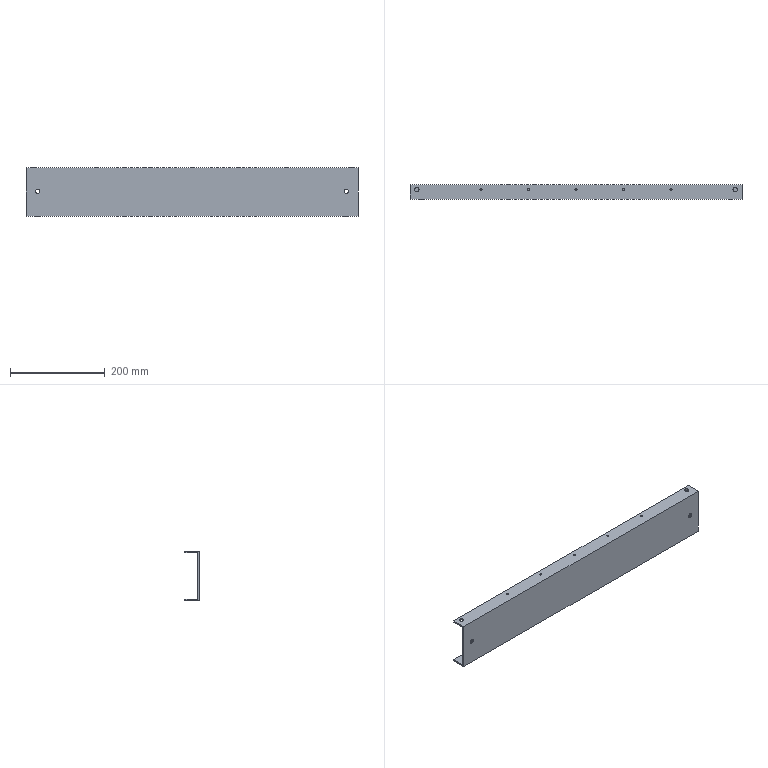Part | SolidWorks | features BaseBody 1 | 1 solid | 32 faces | box 699 x 30 x 103 mm | volume 327650 mm3 | cylinder 22 | plane 10 | commonest cylinder face diameters 4.4 x10 9.1 x8 11 x4
STEP:
#1=CARTESIAN_POINT('',(871.946,-4400.973,890.421));
#2=VERTEX_POINT('',#1);
#3=CARTESIAN_POINT('',(871.946,-4400.973,899.521));
#4=VERTEX_POINT('',#3);
#5=CARTESIAN_POINT('',(871.946,-4400.973,894.971));
#6=DIRECTION('',(0.,1.,0.));
#7=DIRECTION('',(0.,0.,1.));
#8=AXIS2_PLACEMENT_3D('',#5,#6,#7);
#9=CIRCLE('',#8,4.55);
#10=EDGE_CURVE('',#2,#4,#9,.T.);
#11=ORIENTED_EDGE('',*,*,#10,.F.);
#12=CARTESIAN_POINT('',(871.946,-4397.973,890.421));
#13=VERTEX_POINT('',#12);
#14=CARTESIAN_POINT('',(871.946,-4381.737,890.421));
#15=DIRECTION('',(0.,1.,0.));
#16=VECTOR('',#15,1000.);
#17=LINE('',#14,#16);
#18=EDGE_CURVE('',#2,#13,#17,.T.);
#19=ORIENTED_EDGE('',*,*,#18,.T.);
#20=CARTESIAN_POINT('',(871.946,-4397.973,899.521));
#21=VERTEX_POINT('',#20);
#22=CARTESIAN_POINT('',(871.946,-4397.973,894.971));
#23=DIRECTION('',(0.,-1.,0.));
#24=DIRECTION('',(0.,0.,1.));
#25=AXIS2_PLACEMENT_3D('',#22,#23,#24);
#26=CIRCLE('',#25,4.55);
#27=EDGE_CURVE('',#21,#13,#26,.T.);
#28=ORIENTED_EDGE('',*,*,#27,.F.);
#29=CARTESIAN_POINT('',(871.946,-4381.737,899.521));
#30=DIRECTION('',(0.,1.,0.));
#31=VECTOR('',#30,1000.);
#32=LINE('',#29,#31);
#33=EDGE_CURVE('',#4,#21,#32,.T.);
#34=ORIENTED_EDGE('',*,*,#33,.F.);
#35=EDGE_LOOP('',(#11,#19,#28,#34));
#36=FACE_OUTER_BOUND('',#35,.T.);
#37=CARTESIAN_POINT('',(871.946,-4381.737,894.971));
#38=DIRECTION('',(0.,1.,0.));
#39=DIRECTION('',(0.,0.,1.));
#40=AXIS2_PLACEMENT_3D('',#37,#38,#39);
#41=CYLINDRICAL_SURFACE('',#40,4.55);
#42=ADVANCED_FACE('',(#36),#41,.F.);
#43=CARTESIAN_POINT('',(221.946,-4397.973,899.521));
#44=VERTEX_POINT('',#43);
#45=CARTESIAN_POINT('',(221.946,-4397.973,890.421));
#46=VERTEX_POINT('',#45);
#47=CARTESIAN_POINT('',(221.946,-4397.973,894.971));
#48=DIRECTION('',(0.,-1.,0.));
#49=DIRECTION('',(0.,0.,-1.));
#50=AXIS2_PLACEMENT_3D('',#47,#48,#49);
#51=CIRCLE('',#50,4.55);
#52=EDGE_CURVE('',#44,#46,#51,.T.);
#53=ORIENTED_EDGE('',*,*,#52,.F.);
#54=CARTESIAN_POINT('',(221.946,-4400.973,899.521));
#55=VERTEX_POINT('',#54);
#56=CARTESIAN_POINT('',(221.946,-4381.737,899.521));
#57=DIRECTION('',(0.,-1.,0.));
#58=VECTOR('',#57,1000.);
#59=LINE('',#56,#58);
#60=EDGE_CURVE('',#44,#55,#59,.T.);
#61=ORIENTED_EDGE('',*,*,#60,.T.);
#62=CARTESIAN_POINT('',(221.946,-4400.973,890.421));
#63=VERTEX_POINT('',#62);
#64=CARTESIAN_POINT('',(221.946,-4400.973,894.971));
#65=DIRECTION('',(0.,1.,0.));
#66=DIRECTION('',(0.,0.,-1.));
#67=AXIS2_PLACEMENT_3D('',#64,#65,#66);
#68=CIRCLE('',#67,4.55);
#69=EDGE_CURVE('',#63,#55,#68,.T.);
#70=ORIENTED_EDGE('',*,*,#69,.F.);
#71=CARTESIAN_POINT('',(221.946,-4381.737,890.421));
#72=DIRECTION('',(0.,-1.,0.));
#73=VECTOR('',#72,1000.);
#74=LINE('',#71,#73);
#75=EDGE_CURVE('',#46,#63,#74,.T.);
#76=ORIENTED_EDGE('',*,*,#75,.F.);
#77=EDGE_LOOP('',(#53,#61,#70,#76));
#78=FACE_OUTER_BOUND('',#77,.T.);
#79=CARTESIAN_POINT('',(221.946,-4381.737,894.971));
#80=DIRECTION('',(0.,-1.,0.));
#81=DIRECTION('',(0.,0.,-1.));
#82=AXIS2_PLACEMENT_3D('',#79,#80,#81);
#83=CYLINDRICAL_SURFACE('',#82,4.55);
#84=ADVANCED_FACE('',(#78),#83,.F.);
#85=CARTESIAN_POINT('',(886.496,-4380.973,944.971));
#86=VERTEX_POINT('',#85);
#87=CARTESIAN_POINT('',(877.396,-4380.973,944.971));
#88=VERTEX_POINT('',#87);
#89=CARTESIAN_POINT('',(881.946,-4380.973,944.971));
#90=DIRECTION('',(0.,0.,-1.));
#91=DIRECTION('',(-1.,0.,0.));
#92=AXIS2_PLACEMENT_3D('',#89,#90,#91);
#93=CIRCLE('',#92,4.55);
#94=EDGE_CURVE('',#86,#88,#93,.T.);
#95=ORIENTED_EDGE('',*,*,#94,.F.);
#96=CARTESIAN_POINT('',(886.496,-4380.973,941.971));
#97=VERTEX_POINT('',#96);
#98=CARTESIAN_POINT('',(886.496,-4380.973,946.133));
#99=DIRECTION('',(0.,0.,-1.));
#100=VECTOR('',#99,1000.);
#101=LINE('',#98,#100);
#102=EDGE_CURVE('',#86,#97,#101,.T.);
#103=ORIENTED_EDGE('',*,*,#102,.T.);
#104=CARTESIAN_POINT('',(877.396,-4380.973,941.971));
#105=VERTEX_POINT('',#104);
#106=CARTESIAN_POINT('',(881.946,-4380.973,941.971));
#107=DIRECTION('',(0.,0.,1.));
#108=DIRECTION('',(-1.,0.,0.));
#109=AXIS2_PLACEMENT_3D('',#106,#107,#108);
#110=CIRCLE('',#109,4.55);
#111=EDGE_CURVE('',#105,#97,#110,.T.);
#112=ORIENTED_EDGE('',*,*,#111,.F.);
#113=CARTESIAN_POINT('',(877.396,-4380.973,946.133));
#114=DIRECTION('',(0.,0.,-1.));
#115=VECTOR('',#114,1000.);
#116=LINE('',#113,#115);
#117=EDGE_CURVE('',#88,#105,#116,.T.);
#118=ORIENTED_EDGE('',*,*,#117,.F.);
#119=EDGE_LOOP('',(#95,#103,#112,#118));
#120=FACE_OUTER_BOUND('',#119,.T.);
#121=CARTESIAN_POINT('',(881.946,-4380.973,946.133));
#122=DIRECTION('',(0.,0.,-1.));
#123=DIRECTION('',(-1.,0.,0.));
#124=AXIS2_PLACEMENT_3D('',#121,#122,#123);
#125=CYLINDRICAL_SURFACE('',#124,4.55);
#126=ADVANCED_FACE('',(#120),#125,.F.);
#127=CARTESIAN_POINT('',(207.396,-4380.973,941.971));
#128=VERTEX_POINT('',#127);
#129=CARTESIAN_POINT('',(216.496,-4380.973,941.971));
#130=VERTEX_POINT('',#129);
#131=CARTESIAN_POINT('',(211.946,-4380.973,941.971));
#132=DIRECTION('',(0.,0.,1.));
#133=DIRECTION('',(1.,0.,0.));
#134=AXIS2_PLACEMENT_3D('',#131,#132,#133);
#135=CIRCLE('',#134,4.55);
#136=EDGE_CURVE('',#128,#130,#135,.T.);
#137=ORIENTED_EDGE('',*,*,#136,.F.);
#138=CARTESIAN_POINT('',(207.396,-4380.973,944.971));
#139=VERTEX_POINT('',#138);
#140=CARTESIAN_POINT('',(207.396,-4380.973,946.133));
#141=DIRECTION('',(0.,0.,1.));
#142=VECTOR('',#141,1000.);
#143=LINE('',#140,#142);
#144=EDGE_CURVE('',#128,#139,#143,.T.);
#145=ORIENTED_EDGE('',*,*,#144,.T.);
#146=CARTESIAN_POINT('',(216.496,-4380.973,944.971));
#147=VERTEX_POINT('',#146);
#148=CARTESIAN_POINT('',(211.946,-4380.973,944.971));
#149=DIRECTION('',(0.,0.,-1.));
#150=DIRECTION('',(1.,0.,0.));
#151=AXIS2_PLACEMENT_3D('',#148,#149,#150);
#152=CIRCLE('',#151,4.55);
#153=EDGE_CURVE('',#147,#139,#152,.T.);
#154=ORIENTED_EDGE('',*,*,#153,.F.);
#155=CARTESIAN_POINT('',(216.496,-4380.973,946.133));
#156=DIRECTION('',(0.,0.,1.));
#157=VECTOR('',#156,1000.);
#158=LINE('',#155,#157);
#159=EDGE_CURVE('',#130,#147,#158,.T.);
#160=ORIENTED_EDGE('',*,*,#159,.F.);
#161=EDGE_LOOP('',(#137,#145,#154,#160));
#162=FACE_OUTER_BOUND('',#161,.T.);
#163=CARTESIAN_POINT('',(211.946,-4380.973,946.133));
#164=DIRECTION('',(0.,0.,1.));
#165=DIRECTION('',(1.,0.,0.));
#166=AXIS2_PLACEMENT_3D('',#163,#164,#165);
#167=CYLINDRICAL_SURFACE('',#166,4.55);
#168=ADVANCED_FACE('',(#162),#167,.F.);
#169=CARTESIAN_POINT('',(544.746,-4380.973,941.971));
#170=VERTEX_POINT('',#169);
#171=CARTESIAN_POINT('',(549.146,-4380.973,941.971));
#172=VERTEX_POINT('',#171);
#173=CARTESIAN_POINT('',(546.946,-4380.973,941.971));
#174=DIRECTION('',(0.,0.,1.));
#175=DIRECTION('',(1.,0.,0.));
#176=AXIS2_PLACEMENT_3D('',#173,#174,#175);
#177=CIRCLE('',#176,2.2);
#178=EDGE_CURVE('',#170,#172,#177,.T.);
#179=ORIENTED_EDGE('',*,*,#178,.F.);
#180=CARTESIAN_POINT('',(544.746,-4380.973,944.971));
#181=VERTEX_POINT('',#180);
#182=CARTESIAN_POINT('',(544.746,-4380.973,945.024));
#183=DIRECTION('',(0.,0.,1.));
#184=VECTOR('',#183,1000.);
#185=LINE('',#182,#184);
#186=EDGE_CURVE('',#170,#181,#185,.T.);
#187=ORIENTED_EDGE('',*,*,#186,.T.);
#188=CARTESIAN_POINT('',(549.146,-4380.973,944.971));
#189=VERTEX_POINT('',#188);
#190=CARTESIAN_POINT('',(546.946,-4380.973,944.971));
#191=DIRECTION('',(0.,0.,-1.));
#192=DIRECTION('',(1.,0.,0.));
#193=AXIS2_PLACEMENT_3D('',#190,#191,#192);
#194=CIRCLE('',#193,2.2);
#195=EDGE_CURVE('',#189,#181,#194,.T.);
#196=ORIENTED_EDGE('',*,*,#195,.F.);
#197=CARTESIAN_POINT('',(549.146,-4380.973,945.024));
#198=DIRECTION('',(0.,0.,1.));
#199=VECTOR('',#198,1000.);
#200=LINE('',#197,#199);
#201=EDGE_CURVE('',#172,#189,#200,.T.);
#202=ORIENTED_EDGE('',*,*,#201,.F.);
#203=EDGE_LOOP('',(#179,#187,#196,#202));
#204=FACE_OUTER_BOUND('',#203,.T.);
#205=CARTESIAN_POINT('',(546.946,-4380.973,945.024));
#206=DIRECTION('',(0.,0.,1.));
#207=DIRECTION('',(1.,0.,0.));
#208=AXIS2_PLACEMENT_3D('',#205,#206,#207);
#209=CYLINDRICAL_SURFACE('',#208,2.2);
#210=ADVANCED_FACE('',(#204),#209,.F.);
#211=CARTESIAN_POINT('',(344.746,-4380.973,941.971));
#212=VERTEX_POINT('',#211);
#213=CARTESIAN_POINT('',(349.146,-4380.973,941.971));
#214=VERTEX_POINT('',#213);
#215=CARTESIAN_POINT('',(346.946,-4380.973,941.971));
#216=DIRECTION('',(0.,0.,1.));
#217=DIRECTION('',(1.,0.,0.));
#218=AXIS2_PLACEMENT_3D('',#215,#216,#217);
#219=CIRCLE('',#218,2.2);
#220=EDGE_CURVE('',#212,#214,#219,.T.);
#221=ORIENTED_EDGE('',*,*,#220,.F.);
#222=CARTESIAN_POINT('',(344.746,-4380.973,944.971));
#223=VERTEX_POINT('',#222);
#224=CARTESIAN_POINT('',(344.746,-4380.973,945.024));
#225=DIRECTION('',(0.,0.,1.));
#226=VECTOR('',#225,1000.);
#227=LINE('',#224,#226);
#228=EDGE_CURVE('',#212,#223,#227,.T.);
#229=ORIENTED_EDGE('',*,*,#228,.T.);
#230=CARTESIAN_POINT('',(349.146,-4380.973,944.971));
#231=VERTEX_POINT('',#230);
#232=CARTESIAN_POINT('',(346.946,-4380.973,944.971));
#233=DIRECTION('',(0.,0.,-1.));
#234=DIRECTION('',(1.,0.,0.));
#235=AXIS2_PLACEMENT_3D('',#232,#233,#234);
#236=CIRCLE('',#235,2.2);
#237=EDGE_CURVE('',#231,#223,#236,.T.);
#238=ORIENTED_EDGE('',*,*,#237,.F.);
#239=CARTESIAN_POINT('',(349.146,-4380.973,945.024));
#240=DIRECTION('',(0.,0.,1.));
#241=VECTOR('',#240,1000.);
#242=LINE('',#239,#241);
#243=EDGE_CURVE('',#214,#231,#242,.T.);
#244=ORIENTED_EDGE('',*,*,#243,.F.);
#245=EDGE_LOOP('',(#221,#229,#238,#244));
#246=FACE_OUTER_BOUND('',#245,.T.);
#247=CARTESIAN_POINT('',(346.946,-4380.973,945.024));
#248=DIRECTION('',(0.,0.,1.));
#249=DIRECTION('',(1.,0.,0.));
#250=AXIS2_PLACEMENT_3D('',#247,#248,#249);
#251=CYLINDRICAL_SURFACE('',#250,2.2);
#252=ADVANCED_FACE('',(#246),#251,.F.);
#253=CARTESIAN_POINT('',(649.146,-4380.973,944.971));
#254=VERTEX_POINT('',#253);
#255=CARTESIAN_POINT('',(644.746,-4380.973,944.971));
#256=VERTEX_POINT('',#255);
#257=CARTESIAN_POINT('',(646.946,-4380.973,944.971));
#258=DIRECTION('',(0.,0.,-1.));
#259=DIRECTION('',(-1.,0.,0.));
#260=AXIS2_PLACEMENT_3D('',#257,#258,#259);
#261=CIRCLE('',#260,2.2);
#262=EDGE_CURVE('',#254,#256,#261,.T.);
#263=ORIENTED_EDGE('',*,*,#262,.F.);
#264=CARTESIAN_POINT('',(649.146,-4380.973,941.971));
#265=VERTEX_POINT('',#264);
#266=CARTESIAN_POINT('',(649.146,-4380.973,945.024));
#267=DIRECTION('',(0.,0.,-1.));
#268=VECTOR('',#267,1000.);
#269=LINE('',#266,#268);
#270=EDGE_CURVE('',#254,#265,#269,.T.);
#271=ORIENTED_EDGE('',*,*,#270,.T.);
#272=CARTESIAN_POINT('',(644.746,-4380.973,941.971));
#273=VERTEX_POINT('',#272);
#274=CARTESIAN_POINT('',(646.946,-4380.973,941.971));
#275=DIRECTION('',(0.,0.,1.));
#276=DIRECTION('',(-1.,0.,0.));
#277=AXIS2_PLACEMENT_3D('',#274,#275,#276);
#278=CIRCLE('',#277,2.2);
#279=EDGE_CURVE('',#273,#265,#278,.T.);
#280=ORIENTED_EDGE('',*,*,#279,.F.);
#281=CARTESIAN_POINT('',(644.746,-4380.973,945.024));
#282=DIRECTION('',(0.,0.,-1.));
#283=VECTOR('',#282,1000.);
#284=LINE('',#281,#283);
#285=EDGE_CURVE('',#256,#273,#284,.T.);
#286=ORIENTED_EDGE('',*,*,#285,.F.);
#287=EDGE_LOOP('',(#263,#271,#280,#286));
#288=FACE_OUTER_BOUND('',#287,.T.);
#289=CARTESIAN_POINT('',(646.946,-4380.973,945.024));
#290=DIRECTION('',(0.,0.,-1.));
#291=DIRECTION('',(-1.,0.,0.));
#292=AXIS2_PLACEMENT_3D('',#289,#290,#291);
#293=CYLINDRICAL_SURFACE('',#292,2.2);
#294=ADVANCED_FACE('',(#288),#293,.F.);
#295=CARTESIAN_POINT('',(749.146,-4380.973,944.971));
#296=VERTEX_POINT('',#295);
#297=CARTESIAN_POINT('',(744.746,-4380.973,944.971));
#298=VERTEX_POINT('',#297);
#299=CARTESIAN_POINT('',(746.946,-4380.973,944.971));
#300=DIRECTION('',(0.,0.,-1.));
#301=DIRECTION('',(-1.,0.,0.));
#302=AXIS2_PLACEMENT_3D('',#299,#300,#301);
#303=CIRCLE('',#302,2.2);
#304=EDGE_CURVE('',#296,#298,#303,.T.);
#305=ORIENTED_EDGE('',*,*,#304,.F.);
#306=CARTESIAN_POINT('',(749.146,-4380.973,941.971));
#307=VERTEX_POINT('',#306);
#308=CARTESIAN_POINT('',(749.146,-4380.973,945.024));
#309=DIRECTION('',(0.,0.,-1.));
#310=VECTOR('',#309,1000.);
#311=LINE('',#308,#310);
#312=EDGE_CURVE('',#296,#307,#311,.T.);
#313=ORIENTED_EDGE('',*,*,#312,.T.);
#314=CARTESIAN_POINT('',(744.746,-4380.973,941.971));
#315=VERTEX_POINT('',#314);
#316=CARTESIAN_POINT('',(746.946,-4380.973,941.971));
#317=DIRECTION('',(0.,0.,1.));
#318=DIRECTION('',(-1.,0.,0.));
#319=AXIS2_PLACEMENT_3D('',#316,#317,#318);
#320=CIRCLE('',#319,2.2);
#321=EDGE_CURVE('',#315,#307,#320,.T.);
#322=ORIENTED_EDGE('',*,*,#321,.F.);
#323=CARTESIAN_POINT('',(744.746,-4380.973,945.024));
#324=DIRECTION('',(0.,0.,-1.));
#325=VECTOR('',#324,1000.);
#326=LINE('',#323,#325);
#327=EDGE_CURVE('',#298,#315,#326,.T.);
#328=ORIENTED_EDGE('',*,*,#327,.F.);
#329=EDGE_LOOP('',(#305,#313,#322,#328));
#330=FACE_OUTER_BOUND('',#329,.T.);
#331=CARTESIAN_POINT('',(746.946,-4380.973,945.024));
#332=DIRECTION('',(0.,0.,-1.));
#333=DIRECTION('',(-1.,0.,0.));
#334=AXIS2_PLACEMENT_3D('',#331,#332,#333);
#335=CYLINDRICAL_SURFACE('',#334,2.2);
#336=ADVANCED_FACE('',(#330),#335,.F.);
#337=CARTESIAN_POINT('',(444.746,-4380.973,941.971));
#338=VERTEX_POINT('',#337);
#339=CARTESIAN_POINT('',(449.146,-4380.973,941.971));
#340=VERTEX_POINT('',#339);
#341=CARTESIAN_POINT('',(446.946,-4380.973,941.971));
#342=DIRECTION('',(0.,0.,1.));
#343=DIRECTION('',(1.,0.,0.));
#344=AXIS2_PLACEMENT_3D('',#341,#342,#343);
#345=CIRCLE('',#344,2.2);
#346=EDGE_CURVE('',#338,#340,#345,.T.);
#347=ORIENTED_EDGE('',*,*,#346,.F.);
#348=CARTESIAN_POINT('',(444.746,-4380.973,944.971));
#349=VERTEX_POINT('',#348);
#350=CARTESIAN_POINT('',(444.746,-4380.973,945.024));
#351=DIRECTION('',(0.,0.,1.));
#352=VECTOR('',#351,1000.);
#353=LINE('',#350,#352);
#354=EDGE_CURVE('',#338,#349,#353,.T.);
#355=ORIENTED_EDGE('',*,*,#354,.T.);
#356=CARTESIAN_POINT('',(449.146,-4380.973,944.971));
#357=VERTEX_POINT('',#356);
#358=CARTESIAN_POINT('',(446.946,-4380.973,944.971));
#359=DIRECTION('',(0.,0.,-1.));
#360=DIRECTION('',(1.,0.,0.));
#361=AXIS2_PLACEMENT_3D('',#358,#359,#360);
#362=CIRCLE('',#361,2.2);
#363=EDGE_CURVE('',#357,#349,#362,.T.);
#364=ORIENTED_EDGE('',*,*,#363,.F.);
#365=CARTESIAN_POINT('',(449.146,-4380.973,945.024));
#366=DIRECTION('',(0.,0.,1.));
#367=VECTOR('',#366,1000.);
#368=LINE('',#365,#367);
#369=EDGE_CURVE('',#340,#357,#368,.T.);
#370=ORIENTED_EDGE('',*,*,#369,.F.);
#371=EDGE_LOOP('',(#347,#355,#364,#370));
#372=FACE_OUTER_BOUND('',#371,.T.);
#373=CARTESIAN_POINT('',(446.946,-4380.973,945.024));
#374=DIRECTION('',(0.,0.,1.));
#375=DIRECTION('',(1.,0.,0.));
#376=AXIS2_PLACEMENT_3D('',#373,#374,#375);
#377=CYLINDRICAL_SURFACE('',#376,2.2);
#378=ADVANCED_FACE('',(#372),#377,.F.);
#379=CARTESIAN_POINT('',(216.446,-4380.973,841.971));
#380=VERTEX_POINT('',#379);
#381=CARTESIAN_POINT('',(227.446,-4380.973,841.971));
#382=VERTEX_POINT('',#381);
#383=CARTESIAN_POINT('',(221.946,-4380.973,841.971));
#384=DIRECTION('',(0.,0.,1.));
#385=DIRECTION('',(1.,0.,0.));
#386=AXIS2_PLACEMENT_3D('',#383,#384,#385);
#387=CIRCLE('',#386,5.5);
#388=EDGE_CURVE('',#380,#382,#387,.T.);
#389=ORIENTED_EDGE('',*,*,#388,.F.);
#390=CARTESIAN_POINT('',(216.446,-4380.973,844.971));
#391=VERTEX_POINT('',#390);
#392=CARTESIAN_POINT('',(216.446,-4380.973,832.653));
#393=DIRECTION('',(0.,0.,1.));
#394=VECTOR('',#393,1000.);
#395=LINE('',#392,#394);
#396=EDGE_CURVE('',#380,#391,#395,.T.);
#397=ORIENTED_EDGE('',*,*,#396,.T.);
#398=CARTESIAN_POINT('',(227.446,-4380.973,844.971));
#399=VERTEX_POINT('',#398);
#400=CARTESIAN_POINT('',(221.946,-4380.973,844.971));
#401=DIRECTION('',(0.,0.,-1.));
#402=DIRECTION('',(1.,0.,0.));
#403=AXIS2_PLACEMENT_3D('',#400,#401,#402);
#404=CIRCLE('',#403,5.5);
#405=EDGE_CURVE('',#399,#391,#404,.T.);
#406=ORIENTED_EDGE('',*,*,#405,.F.);
#407=CARTESIAN_POINT('',(227.446,-4380.973,832.653));
#408=DIRECTION('',(0.,0.,1.));
#409=VECTOR('',#408,1000.);
#410=LINE('',#407,#409);
#411=EDGE_CURVE('',#382,#399,#410,.T.);
#412=ORIENTED_EDGE('',*,*,#411,.F.);
#413=EDGE_LOOP('',(#389,#397,#406,#412));
#414=FACE_OUTER_BOUND('',#413,.T.);
#415=CARTESIAN_POINT('',(221.946,-4380.973,832.653));
#416=DIRECTION('',(0.,0.,1.));
#417=DIRECTION('',(1.,0.,0.));
#418=AXIS2_PLACEMENT_3D('',#415,#416,#417);
#419=CYLINDRICAL_SURFACE('',#418,5.5);
#420=ADVANCED_FACE('',(#414),#419,.F.);
#421=CARTESIAN_POINT('',(877.446,-4380.973,844.971));
#422=VERTEX_POINT('',#421);
#423=CARTESIAN_POINT('',(866.446,-4380.973,844.971));
#424=VERTEX_POINT('',#423);
#425=CARTESIAN_POINT('',(871.946,-4380.973,844.971));
#426=DIRECTION('',(0.,0.,-1.));
#427=DIRECTION('',(-1.,0.,0.));
#428=AXIS2_PLACEMENT_3D('',#425,#426,#427);
#429=CIRCLE('',#428,5.5);
#430=EDGE_CURVE('',#422,#424,#429,.T.);
#431=ORIENTED_EDGE('',*,*,#430,.F.);
#432=CARTESIAN_POINT('',(877.446,-4380.973,841.971));
#433=VERTEX_POINT('',#432);
#434=CARTESIAN_POINT('',(877.446,-4380.973,832.653));
#435=DIRECTION('',(0.,0.,-1.));
#436=VECTOR('',#435,1000.);
#437=LINE('',#434,#436);
#438=EDGE_CURVE('',#422,#433,#437,.T.);
#439=ORIENTED_EDGE('',*,*,#438,.T.);
#440=CARTESIAN_POINT('',(866.446,-4380.973,841.971));
#441=VERTEX_POINT('',#440);
#442=CARTESIAN_POINT('',(871.946,-4380.973,841.971));
#443=DIRECTION('',(0.,0.,1.));
#444=DIRECTION('',(-1.,0.,0.));
#445=AXIS2_PLACEMENT_3D('',#442,#443,#444);
#446=CIRCLE('',#445,5.5);
#447=EDGE_CURVE('',#441,#433,#446,.T.);
#448=ORIENTED_EDGE('',*,*,#447,.F.);
#449=CARTESIAN_POINT('',(866.446,-4380.973,832.653));
#450=DIRECTION('',(0.,0.,-1.));
#451=VECTOR('',#450,1000.);
#452=LINE('',#449,#451);
#453=EDGE_CURVE('',#424,#441,#452,.T.);
#454=ORIENTED_EDGE('',*,*,#453,.F.);
#455=EDGE_LOOP('',(#431,#439,#448,#454));
#456=FACE_OUTER_BOUND('',#455,.T.);
#457=CARTESIAN_POINT('',(871.946,-4380.973,832.653));
#458=DIRECTION('',(0.,0.,-1.));
#459=DIRECTION('',(-1.,0.,0.));
#460=AXIS2_PLACEMENT_3D('',#457,#458,#459);
#461=CYLINDRICAL_SURFACE('',#460,5.5);
#462=ADVANCED_FACE('',(#456),#461,.F.);
#463=CARTESIAN_POINT('',(896.446,-4400.973,841.971));
#464=VERTEX_POINT('',#463);
#465=CARTESIAN_POINT('',(896.446,-4400.973,944.971));
#466=VERTEX_POINT('',#465);
#467=CARTESIAN_POINT('',(896.446,-4400.973,944.971));
#468=DIRECTION('',(0.,0.,1.));
#469=VECTOR('',#468,1000.);
#470=LINE('',#467,#469);
#471=EDGE_CURVE('',#464,#466,#470,.T.);
#472=ORIENTED_EDGE('',*,*,#471,.T.);
#473=CARTESIAN_POINT('',(197.446,-4400.973,944.971));
#474=VERTEX_POINT('',#473);
#475=CARTESIAN_POINT('',(896.446,-4400.973,944.971));
#476=DIRECTION('',(-1.,0.,0.));
#477=VECTOR('',#476,1000.);
#478=LINE('',#475,#477);
#479=EDGE_CURVE('',#466,#474,#478,.T.);
#480=ORIENTED_EDGE('',*,*,#479,.T.);
#481=CARTESIAN_POINT('',(197.446,-4400.973,841.971));
#482=VERTEX_POINT('',#481);
#483=CARTESIAN_POINT('',(197.446,-4400.973,944.971));
#484=DIRECTION('',(0.,0.,-1.));
#485=VECTOR('',#484,1000.);
#486=LINE('',#483,#485);
#487=EDGE_CURVE('',#474,#482,#486,.T.);
#488=ORIENTED_EDGE('',*,*,#487,.T.);
#489=CARTESIAN_POINT('',(896.446,-4400.973,841.971));
#490=DIRECTION('',(1.,0.,0.));
#491=VECTOR('',#490,1000.);
#492=LINE('',#489,#491);
#493=EDGE_CURVE('',#482,#464,#492,.T.);
#494=ORIENTED_EDGE('',*,*,#493,.T.);
#495=EDGE_LOOP('',(#472,#480,#488,#494));
#496=FACE_OUTER_BOUND('',#495,.T.);
#497=CARTESIAN_POINT('',(871.946,-4400.973,894.971));
#498=DIRECTION('',(0.,1.,0.));
#499=DIRECTION('',(0.,0.,1.));
#500=AXIS2_PLACEMENT_3D('',#497,#498,#499);
#501=CIRCLE('',#500,4.55);
#502=EDGE_CURVE('',#4,#2,#501,.T.);
#503=ORIENTED_EDGE('',*,*,#502,.T.);
#504=ORIENTED_EDGE('',*,*,#10,.T.);
#505=EDGE_LOOP('',(#503,#504));
#506=FACE_BOUND('',#505,.T.);
#507=ORIENTED_EDGE('',*,*,#69,.T.);
#508=CARTESIAN_POINT('',(221.946,-4400.973,894.971));
#509=DIRECTION('',(0.,1.,0.));
#510=DIRECTION('',(0.,0.,-1.));
#511=AXIS2_PLACEMENT_3D('',#508,#509,#510);
#512=CIRCLE('',#511,4.55);
#513=EDGE_CURVE('',#55,#63,#512,.T.);
#514=ORIENTED_EDGE('',*,*,#513,.T.);
#515=EDGE_LOOP('',(#507,#514));
#516=FACE_BOUND('',#515,.T.);
#517=CARTESIAN_POINT('',(896.446,-4400.973,944.971));
#518=DIRECTION('',(0.,-1.,0.));
#519=DIRECTION('',(0.,0.,-1.));
#520=AXIS2_PLACEMENT_3D('',#517,#518,#519);
#521=PLANE('',#520);
#522=ADVANCED_FACE('',(#496,#506,#516),#521,.T.);
#523=CARTESIAN_POINT('',(896.446,-4370.973,944.971));
#524=VERTEX_POINT('',#523);
#525=CARTESIAN_POINT('',(896.446,-4375.973,944.971));
#526=DIRECTION('',(0.,1.,0.));
#527=VECTOR('',#526,1000.);
#528=LINE('',#525,#527);
#529=EDGE_CURVE('',#466,#524,#528,.T.);
#530=ORIENTED_EDGE('',*,*,#529,.T.);
#531=CARTESIAN_POINT('',(197.446,-4370.973,944.971));
#532=VERTEX_POINT('',#531);
#533=CARTESIAN_POINT('',(896.446,-4370.973,944.971));
#534=DIRECTION('',(-1.,0.,0.));
#535=VECTOR('',#534,1000.);
#536=LINE('',#533,#535);
#537=EDGE_CURVE('',#524,#532,#536,.T.);
#538=ORIENTED_EDGE('',*,*,#537,.T.);
#539=CARTESIAN_POINT('',(197.446,-4375.973,944.971));
#540=DIRECTION('',(0.,-1.,0.));
#541=VECTOR('',#540,1000.);
#542=LINE('',#539,#541);
#543=EDGE_CURVE('',#532,#474,#542,.T.);
#544=ORIENTED_EDGE('',*,*,#543,.T.);
#545=ORIENTED_EDGE('',*,*,#479,.F.);
#546=EDGE_LOOP('',(#530,#538,#544,#545));
#547=FACE_OUTER_BOUND('',#546,.T.);
#548=CARTESIAN_POINT('',(881.946,-4380.973,944.971));
#549=DIRECTION('',(0.,0.,-1.));
#550=DIRECTION('',(-1.,0.,0.));
#551=AXIS2_PLACEMENT_3D('',#548,#549,#550);
#552=CIRCLE('',#551,4.55);
#553=EDGE_CURVE('',#88,#86,#552,.T.);
#554=ORIENTED_EDGE('',*,*,#553,.T.);
#555=ORIENTED_EDGE('',*,*,#94,.T.);
#556=EDGE_LOOP('',(#554,#555));
#557=FACE_BOUND('',#556,.T.);
#558=ORIENTED_EDGE('',*,*,#153,.T.);
#559=CARTESIAN_POINT('',(211.946,-4380.973,944.971));
#560=DIRECTION('',(0.,0.,-1.));
#561=DIRECTION('',(1.,0.,0.));
#562=AXIS2_PLACEMENT_3D('',#559,#560,#561);
#563=CIRCLE('',#562,4.55);
#564=EDGE_CURVE('',#139,#147,#563,.T.);
#565=ORIENTED_EDGE('',*,*,#564,.T.);
#566=EDGE_LOOP('',(#558,#565));
#567=FACE_BOUND('',#566,.T.);
#568=ORIENTED_EDGE('',*,*,#195,.T.);
#569=CARTESIAN_POINT('',(546.946,-4380.973,944.971));
#570=DIRECTION('',(0.,0.,-1.));
#571=DIRECTION('',(1.,0.,0.));
#572=AXIS2_PLACEMENT_3D('',#569,#570,#571);
#573=CIRCLE('',#572,2.2);
#574=EDGE_CURVE('',#181,#189,#573,.T.);
#575=ORIENTED_EDGE('',*,*,#574,.T.);
#576=EDGE_LOOP('',(#568,#575));
#577=FACE_BOUND('',#576,.T.);
#578=ORIENTED_EDGE('',*,*,#237,.T.);
#579=CARTESIAN_POINT('',(346.946,-4380.973,944.971));
#580=DIRECTION('',(0.,0.,-1.));
#581=DIRECTION('',(1.,0.,0.));
#582=AXIS2_PLACEMENT_3D('',#579,#580,#581);
#583=CIRCLE('',#582,2.2);
#584=EDGE_CURVE('',#223,#231,#583,.T.);
#585=ORIENTED_EDGE('',*,*,#584,.T.);
#586=EDGE_LOOP('',(#578,#585));
#587=FACE_BOUND('',#586,.T.);
#588=CARTESIAN_POINT('',(646.946,-4380.973,944.971));
#589=DIRECTION('',(0.,0.,-1.));
#590=DIRECTION('',(-1.,0.,0.));
#591=AXIS2_PLACEMENT_3D('',#588,#589,#590);
#592=CIRCLE('',#591,2.2);
#593=EDGE_CURVE('',#256,#254,#592,.T.);
#594=ORIENTED_EDGE('',*,*,#593,.T.);
#595=ORIENTED_EDGE('',*,*,#262,.T.);
#596=EDGE_LOOP('',(#594,#595));
#597=FACE_BOUND('',#596,.T.);
#598=CARTESIAN_POINT('',(746.946,-4380.973,944.971));
#599=DIRECTION('',(0.,0.,-1.));
#600=DIRECTION('',(-1.,0.,0.));
#601=AXIS2_PLACEMENT_3D('',#598,#599,#600);
#602=CIRCLE('',#601,2.2);
#603=EDGE_CURVE('',#298,#296,#602,.T.);
#604=ORIENTED_EDGE('',*,*,#603,.T.);
#605=ORIENTED_EDGE('',*,*,#304,.T.);
#606=EDGE_LOOP('',(#604,#605));
#607=FACE_BOUND('',#606,.T.);
#608=ORIENTED_EDGE('',*,*,#363,.T.);
#609=CARTESIAN_POINT('',(446.946,-4380.973,944.971));
#610=DIRECTION('',(0.,0.,-1.));
#611=DIRECTION('',(1.,0.,0.));
#612=AXIS2_PLACEMENT_3D('',#609,#610,#611);
#613=CIRCLE('',#612,2.2);
#614=EDGE_CURVE('',#349,#357,#613,.T.);
#615=ORIENTED_EDGE('',*,*,#614,.T.);
#616=EDGE_LOOP('',(#608,#615));
#617=FACE_BOUND('',#616,.T.);
#618=CARTESIAN_POINT('',(896.446,-4375.973,944.971));
#619=DIRECTION('',(0.,0.,1.));
#620=DIRECTION('',(1.,0.,0.));
#621=AXIS2_PLACEMENT_3D('',#618,#619,#620);
#622=PLANE('',#621);
#623=ADVANCED_FACE('',(#547,#557,#567,#577,#587,#597,#607,#617),#622,.T.);
#624=CARTESIAN_POINT('',(896.446,-4397.973,844.971));
#625=VERTEX_POINT('',#624);
#626=CARTESIAN_POINT('',(896.446,-4397.973,941.971));
#627=VERTEX_POINT('',#626);
#628=CARTESIAN_POINT('',(896.446,-4397.973,901.99));
#629=DIRECTION('',(0.,0.,1.));
#630=VECTOR('',#629,1000.);
#631=LINE('',#628,#630);
#632=EDGE_CURVE('',#625,#627,#631,.T.);
#633=ORIENTED_EDGE('',*,*,#632,.T.);
#634=CARTESIAN_POINT('',(896.446,-4370.973,941.971));
#635=VERTEX_POINT('',#634);
#636=CARTESIAN_POINT('',(896.446,-4393.892,941.971));
#637=DIRECTION('',(0.,1.,0.));
#638=VECTOR('',#637,1000.);
#639=LINE('',#636,#638);
#640=EDGE_CURVE('',#627,#635,#639,.T.);
#641=ORIENTED_EDGE('',*,*,#640,.T.);
#642=CARTESIAN_POINT('',(896.446,-4370.973,901.99));
#643=DIRECTION('',(0.,0.,1.));
#644=VECTOR('',#643,1000.);
#645=LINE('',#642,#644);
#646=EDGE_CURVE('',#635,#524,#645,.T.);
#647=ORIENTED_EDGE('',*,*,#646,.T.);
#648=ORIENTED_EDGE('',*,*,#529,.F.);
#649=ORIENTED_EDGE('',*,*,#471,.F.);
#650=CARTESIAN_POINT('',(896.446,-4370.973,841.971));
#651=VERTEX_POINT('',#650);
#652=CARTESIAN_POINT('',(896.446,-4393.892,841.971));
#653=DIRECTION('',(0.,1.,0.));
#654=VECTOR('',#653,1000.);
#655=LINE('',#652,#654);
#656=EDGE_CURVE('',#464,#651,#655,.T.);
#657=ORIENTED_EDGE('',*,*,#656,.T.);
#658=CARTESIAN_POINT('',(896.446,-4370.973,844.971));
#659=VERTEX_POINT('',#658);
#660=CARTESIAN_POINT('',(896.446,-4370.973,901.99));
#661=DIRECTION('',(0.,0.,1.));
#662=VECTOR('',#661,1000.);
#663=LINE('',#660,#662);
#664=EDGE_CURVE('',#651,#659,#663,.T.);
#665=ORIENTED_EDGE('',*,*,#664,.T.);
#666=CARTESIAN_POINT('',(896.446,-4393.892,844.971));
#667=DIRECTION('',(0.,-1.,0.));
#668=VECTOR('',#667,1000.);
#669=LINE('',#666,#668);
#670=EDGE_CURVE('',#659,#625,#669,.T.);
#671=ORIENTED_EDGE('',*,*,#670,.T.);
#672=EDGE_LOOP('',(#633,#641,#647,#648,#649,#657,#665,#671));
#673=FACE_OUTER_BOUND('',#672,.T.);
#674=CARTESIAN_POINT('',(896.446,-4393.892,901.99));
#675=DIRECTION('',(1.,0.,0.));
#676=DIRECTION('',(0.,0.,-1.));
#677=AXIS2_PLACEMENT_3D('',#674,#675,#676);
#678=PLANE('',#677);
#679=ADVANCED_FACE('',(#673),#678,.T.);
#680=ORIENTED_EDGE('',*,*,#656,.F.);
#681=ORIENTED_EDGE('',*,*,#493,.F.);
#682=CARTESIAN_POINT('',(197.446,-4370.973,841.971));
#683=VERTEX_POINT('',#682);
#684=CARTESIAN_POINT('',(197.446,-4400.973,841.971));
#685=DIRECTION('',(0.,1.,0.));
#686=VECTOR('',#685,1000.);
#687=LINE('',#684,#686);
#688=EDGE_CURVE('',#482,#683,#687,.T.);
#689=ORIENTED_EDGE('',*,*,#688,.T.);
#690=CARTESIAN_POINT('',(896.446,-4370.973,841.971));
#691=DIRECTION('',(1.,0.,0.));
#692=VECTOR('',#691,1000.);
#693=LINE('',#690,#692);
#694=EDGE_CURVE('',#683,#651,#693,.T.);
#695=ORIENTED_EDGE('',*,*,#694,.T.);
#696=EDGE_LOOP('',(#680,#681,#689,#695));
#697=FACE_OUTER_BOUND('',#696,.T.);
#698=CARTESIAN_POINT('',(221.946,-4380.973,841.971));
#699=DIRECTION('',(0.,0.,1.));
#700=DIRECTION('',(1.,0.,0.));
#701=AXIS2_PLACEMENT_3D('',#698,#699,#700);
#702=CIRCLE('',#701,5.5);
#703=EDGE_CURVE('',#382,#380,#702,.T.);
#704=ORIENTED_EDGE('',*,*,#703,.T.);
#705=ORIENTED_EDGE('',*,*,#388,.T.);
#706=EDGE_LOOP('',(#704,#705));
#707=FACE_BOUND('',#706,.T.);
#708=ORIENTED_EDGE('',*,*,#447,.T.);
#709=CARTESIAN_POINT('',(871.946,-4380.973,841.971));
#710=DIRECTION('',(0.,0.,1.));
#711=DIRECTION('',(-1.,0.,0.));
#712=AXIS2_PLACEMENT_3D('',#709,#710,#711);
#713=CIRCLE('',#712,5.5);
#714=EDGE_CURVE('',#433,#441,#713,.T.);
#715=ORIENTED_EDGE('',*,*,#714,.T.);
#716=EDGE_LOOP('',(#708,#715));
#717=FACE_BOUND('',#716,.T.);
#718=CARTESIAN_POINT('',(896.446,-4400.973,841.971));
#719=DIRECTION('',(0.,0.,-1.));
#720=DIRECTION('',(-1.,0.,0.));
#721=AXIS2_PLACEMENT_3D('',#718,#719,#720);
#722=PLANE('',#721);
#723=ADVANCED_FACE('',(#697,#707,#717),#722,.T.);
#724=CARTESIAN_POINT('',(197.446,-4370.973,941.971));
#725=VERTEX_POINT('',#724);
#726=CARTESIAN_POINT('',(197.446,-4370.973,901.99));
#727=DIRECTION('',(0.,0.,1.));
#728=VECTOR('',#727,1000.);
#729=LINE('',#726,#728);
#730=EDGE_CURVE('',#725,#532,#729,.T.);
#731=ORIENTED_EDGE('',*,*,#730,.F.);
#732=CARTESIAN_POINT('',(197.446,-4397.973,941.971));
#733=VERTEX_POINT('',#732);
#734=CARTESIAN_POINT('',(197.446,-4393.892,941.971));
#735=DIRECTION('',(0.,1.,0.));
#736=VECTOR('',#735,1000.);
#737=LINE('',#734,#736);
#738=EDGE_CURVE('',#733,#725,#737,.T.);
#739=ORIENTED_EDGE('',*,*,#738,.F.);
#740=CARTESIAN_POINT('',(197.446,-4397.973,844.971));
#741=VERTEX_POINT('',#740);
#742=CARTESIAN_POINT('',(197.446,-4397.973,901.99));
#743=DIRECTION('',(0.,0.,1.));
#744=VECTOR('',#743,1000.);
#745=LINE('',#742,#744);
#746=EDGE_CURVE('',#741,#733,#745,.T.);
#747=ORIENTED_EDGE('',*,*,#746,.F.);
#748=CARTESIAN_POINT('',(197.446,-4370.973,844.971));
#749=VERTEX_POINT('',#748);
#750=CARTESIAN_POINT('',(197.446,-4393.892,844.971));
#751=DIRECTION('',(0.,-1.,0.));
#752=VECTOR('',#751,1000.);
#753=LINE('',#750,#752);
#754=EDGE_CURVE('',#749,#741,#753,.T.);
#755=ORIENTED_EDGE('',*,*,#754,.F.);
#756=CARTESIAN_POINT('',(197.446,-4370.973,901.99));
#757=DIRECTION('',(0.,0.,1.));
#758=VECTOR('',#757,1000.);
#759=LINE('',#756,#758);
#760=EDGE_CURVE('',#683,#749,#759,.T.);
#761=ORIENTED_EDGE('',*,*,#760,.F.);
#762=ORIENTED_EDGE('',*,*,#688,.F.);
#763=ORIENTED_EDGE('',*,*,#487,.F.);
#764=ORIENTED_EDGE('',*,*,#543,.F.);
#765=EDGE_LOOP('',(#731,#739,#747,#755,#761,#762,#763,#764));
#766=FACE_OUTER_BOUND('',#765,.T.);
#767=CARTESIAN_POINT('',(197.446,-4393.892,901.99));
#768=DIRECTION('',(1.,0.,0.));
#769=DIRECTION('',(0.,0.,-1.));
#770=AXIS2_PLACEMENT_3D('',#767,#768,#769);
#771=PLANE('',#770);
#772=ADVANCED_FACE('',(#766),#771,.F.);
#773=ORIENTED_EDGE('',*,*,#18,.F.);
#774=ORIENTED_EDGE('',*,*,#502,.F.);
#775=ORIENTED_EDGE('',*,*,#33,.T.);
#776=CARTESIAN_POINT('',(871.946,-4397.973,894.971));
#777=DIRECTION('',(0.,-1.,0.));
#778=DIRECTION('',(0.,0.,1.));
#779=AXIS2_PLACEMENT_3D('',#776,#777,#778);
#780=CIRCLE('',#779,4.55);
#781=EDGE_CURVE('',#13,#21,#780,.T.);
#782=ORIENTED_EDGE('',*,*,#781,.F.);
#783=EDGE_LOOP('',(#773,#774,#775,#782));
#784=FACE_OUTER_BOUND('',#783,.T.);
#785=CARTESIAN_POINT('',(871.946,-4381.737,894.971));
#786=DIRECTION('',(0.,1.,0.));
#787=DIRECTION('',(0.,0.,1.));
#788=AXIS2_PLACEMENT_3D('',#785,#786,#787);
#789=CYLINDRICAL_SURFACE('',#788,4.55);
#790=ADVANCED_FACE('',(#784),#789,.F.);
#791=ORIENTED_EDGE('',*,*,#60,.F.);
#792=CARTESIAN_POINT('',(221.946,-4397.973,894.971));
#793=DIRECTION('',(0.,-1.,0.));
#794=DIRECTION('',(0.,0.,-1.));
#795=AXIS2_PLACEMENT_3D('',#792,#793,#794);
#796=CIRCLE('',#795,4.55);
#797=EDGE_CURVE('',#46,#44,#796,.T.);
#798=ORIENTED_EDGE('',*,*,#797,.F.);
#799=ORIENTED_EDGE('',*,*,#75,.T.);
#800=ORIENTED_EDGE('',*,*,#513,.F.);
#801=EDGE_LOOP('',(#791,#798,#799,#800));
#802=FACE_OUTER_BOUND('',#801,.T.);
#803=CARTESIAN_POINT('',(221.946,-4381.737,894.971));
#804=DIRECTION('',(0.,-1.,0.));
#805=DIRECTION('',(0.,0.,-1.));
#806=AXIS2_PLACEMENT_3D('',#803,#804,#805);
#807=CYLINDRICAL_SURFACE('',#806,4.55);
#808=ADVANCED_FACE('',(#802),#807,.F.);
#809=ORIENTED_EDGE('',*,*,#646,.F.);
#810=CARTESIAN_POINT('',(896.446,-4370.973,941.971));
#811=DIRECTION('',(-1.,0.,0.));
#812=VECTOR('',#811,1000.);
#813=LINE('',#810,#812);
#814=EDGE_CURVE('',#635,#725,#813,.T.);
#815=ORIENTED_EDGE('',*,*,#814,.T.);
#816=ORIENTED_EDGE('',*,*,#730,.T.);
#817=ORIENTED_EDGE('',*,*,#537,.F.);
#818=EDGE_LOOP('',(#809,#815,#816,#817));
#819=FACE_OUTER_BOUND('',#818,.T.);
#820=CARTESIAN_POINT('',(896.446,-4370.973,941.971));
#821=DIRECTION('',(0.,1.,0.));
#822=DIRECTION('',(0.,0.,1.));
#823=AXIS2_PLACEMENT_3D('',#820,#821,#822);
#824=PLANE('',#823);
#825=ADVANCED_FACE('',(#819),#824,.T.);
#826=ORIENTED_EDGE('',*,*,#102,.F.);
#827=ORIENTED_EDGE('',*,*,#553,.F.);
#828=ORIENTED_EDGE('',*,*,#117,.T.);
#829=CARTESIAN_POINT('',(881.946,-4380.973,941.971));
#830=DIRECTION('',(0.,0.,1.));
#831=DIRECTION('',(-1.,0.,0.));
#832=AXIS2_PLACEMENT_3D('',#829,#830,#831);
#833=CIRCLE('',#832,4.55);
#834=EDGE_CURVE('',#97,#105,#833,.T.);
#835=ORIENTED_EDGE('',*,*,#834,.F.);
#836=EDGE_LOOP('',(#826,#827,#828,#835));
#837=FACE_OUTER_BOUND('',#836,.T.);
#838=CARTESIAN_POINT('',(881.946,-4380.973,946.133));
#839=DIRECTION('',(0.,0.,-1.));
#840=DIRECTION('',(-1.,0.,0.));
#841=AXIS2_PLACEMENT_3D('',#838,#839,#840);
#842=CYLINDRICAL_SURFACE('',#841,4.55);
#843=ADVANCED_FACE('',(#837),#842,.F.);
#844=ORIENTED_EDGE('',*,*,#144,.F.);
#845=CARTESIAN_POINT('',(211.946,-4380.973,941.971));
#846=DIRECTION('',(0.,0.,1.));
#847=DIRECTION('',(1.,0.,0.));
#848=AXIS2_PLACEMENT_3D('',#845,#846,#847);
#849=CIRCLE('',#848,4.55);
#850=EDGE_CURVE('',#130,#128,#849,.T.);
#851=ORIENTED_EDGE('',*,*,#850,.F.);
#852=ORIENTED_EDGE('',*,*,#159,.T.);
#853=ORIENTED_EDGE('',*,*,#564,.F.);
#854=EDGE_LOOP('',(#844,#851,#852,#853));
#855=FACE_OUTER_BOUND('',#854,.T.);
#856=CARTESIAN_POINT('',(211.946,-4380.973,946.133));
#857=DIRECTION('',(0.,0.,1.));
#858=DIRECTION('',(1.,0.,0.));
#859=AXIS2_PLACEMENT_3D('',#856,#857,#858);
#860=CYLINDRICAL_SURFACE('',#859,4.55);
#861=ADVANCED_FACE('',(#855),#860,.F.);
#862=ORIENTED_EDGE('',*,*,#186,.F.);
#863=CARTESIAN_POINT('',(546.946,-4380.973,941.971));
#864=DIRECTION('',(0.,0.,1.));
#865=DIRECTION('',(1.,0.,0.));
#866=AXIS2_PLACEMENT_3D('',#863,#864,#865);
#867=CIRCLE('',#866,2.2);
#868=EDGE_CURVE('',#172,#170,#867,.T.);
#869=ORIENTED_EDGE('',*,*,#868,.F.);
#870=ORIENTED_EDGE('',*,*,#201,.T.);
#871=ORIENTED_EDGE('',*,*,#574,.F.);
#872=EDGE_LOOP('',(#862,#869,#870,#871));
#873=FACE_OUTER_BOUND('',#872,.T.);
#874=CARTESIAN_POINT('',(546.946,-4380.973,945.024));
#875=DIRECTION('',(0.,0.,1.));
#876=DIRECTION('',(1.,0.,0.));
#877=AXIS2_PLACEMENT_3D('',#874,#875,#876);
#878=CYLINDRICAL_SURFACE('',#877,2.2);
#879=ADVANCED_FACE('',(#873),#878,.F.);
#880=ORIENTED_EDGE('',*,*,#228,.F.);
#881=CARTESIAN_POINT('',(346.946,-4380.973,941.971));
#882=DIRECTION('',(0.,0.,1.));
#883=DIRECTION('',(1.,0.,0.));
#884=AXIS2_PLACEMENT_3D('',#881,#882,#883);
#885=CIRCLE('',#884,2.2);
#886=EDGE_CURVE('',#214,#212,#885,.T.);
#887=ORIENTED_EDGE('',*,*,#886,.F.);
#888=ORIENTED_EDGE('',*,*,#243,.T.);
#889=ORIENTED_EDGE('',*,*,#584,.F.);
#890=EDGE_LOOP('',(#880,#887,#888,#889));
#891=FACE_OUTER_BOUND('',#890,.T.);
#892=CARTESIAN_POINT('',(346.946,-4380.973,945.024));
#893=DIRECTION('',(0.,0.,1.));
#894=DIRECTION('',(1.,0.,0.));
#895=AXIS2_PLACEMENT_3D('',#892,#893,#894);
#896=CYLINDRICAL_SURFACE('',#895,2.2);
#897=ADVANCED_FACE('',(#891),#896,.F.);
#898=ORIENTED_EDGE('',*,*,#270,.F.);
#899=ORIENTED_EDGE('',*,*,#593,.F.);
#900=ORIENTED_EDGE('',*,*,#285,.T.);
#901=CARTESIAN_POINT('',(646.946,-4380.973,941.971));
#902=DIRECTION('',(0.,0.,1.));
#903=DIRECTION('',(-1.,0.,0.));
#904=AXIS2_PLACEMENT_3D('',#901,#902,#903);
#905=CIRCLE('',#904,2.2);
#906=EDGE_CURVE('',#265,#273,#905,.T.);
#907=ORIENTED_EDGE('',*,*,#906,.F.);
#908=EDGE_LOOP('',(#898,#899,#900,#907));
#909=FACE_OUTER_BOUND('',#908,.T.);
#910=CARTESIAN_POINT('',(646.946,-4380.973,945.024));
#911=DIRECTION('',(0.,0.,-1.));
#912=DIRECTION('',(-1.,0.,0.));
#913=AXIS2_PLACEMENT_3D('',#910,#911,#912);
#914=CYLINDRICAL_SURFACE('',#913,2.2);
#915=ADVANCED_FACE('',(#909),#914,.F.);
#916=ORIENTED_EDGE('',*,*,#312,.F.);
#917=ORIENTED_EDGE('',*,*,#603,.F.);
#918=ORIENTED_EDGE('',*,*,#327,.T.);
#919=CARTESIAN_POINT('',(746.946,-4380.973,941.971));
#920=DIRECTION('',(0.,0.,1.));
#921=DIRECTION('',(-1.,0.,0.));
#922=AXIS2_PLACEMENT_3D('',#919,#920,#921);
#923=CIRCLE('',#922,2.2);
#924=EDGE_CURVE('',#307,#315,#923,.T.);
#925=ORIENTED_EDGE('',*,*,#924,.F.);
#926=EDGE_LOOP('',(#916,#917,#918,#925));
#927=FACE_OUTER_BOUND('',#926,.T.);
#928=CARTESIAN_POINT('',(746.946,-4380.973,945.024));
#929=DIRECTION('',(0.,0.,-1.));
#930=DIRECTION('',(-1.,0.,0.));
#931=AXIS2_PLACEMENT_3D('',#928,#929,#930);
#932=CYLINDRICAL_SURFACE('',#931,2.2);
#933=ADVANCED_FACE('',(#927),#932,.F.);
#934=ORIENTED_EDGE('',*,*,#354,.F.);
#935=CARTESIAN_POINT('',(446.946,-4380.973,941.971));
#936=DIRECTION('',(0.,0.,1.));
#937=DIRECTION('',(1.,0.,0.));
#938=AXIS2_PLACEMENT_3D('',#935,#936,#937);
#939=CIRCLE('',#938,2.2);
#940=EDGE_CURVE('',#340,#338,#939,.T.);
#941=ORIENTED_EDGE('',*,*,#940,.F.);
#942=ORIENTED_EDGE('',*,*,#369,.T.);
#943=ORIENTED_EDGE('',*,*,#614,.F.);
#944=EDGE_LOOP('',(#934,#941,#942,#943));
#945=FACE_OUTER_BOUND('',#944,.T.);
#946=CARTESIAN_POINT('',(446.946,-4380.973,945.024));
#947=DIRECTION('',(0.,0.,1.));
#948=DIRECTION('',(1.,0.,0.));
#949=AXIS2_PLACEMENT_3D('',#946,#947,#948);
#950=CYLINDRICAL_SURFACE('',#949,2.2);
#951=ADVANCED_FACE('',(#945),#950,.F.);
#952=ORIENTED_EDGE('',*,*,#640,.F.);
#953=CARTESIAN_POINT('',(896.446,-4397.973,941.971));
#954=DIRECTION('',(-1.,0.,0.));
#955=VECTOR('',#954,1000.);
#956=LINE('',#953,#955);
#957=EDGE_CURVE('',#627,#733,#956,.T.);
#958=ORIENTED_EDGE('',*,*,#957,.T.);
#959=ORIENTED_EDGE('',*,*,#738,.T.);
#960=ORIENTED_EDGE('',*,*,#814,.F.);
#961=EDGE_LOOP('',(#952,#958,#959,#960));
#962=FACE_OUTER_BOUND('',#961,.T.);
#963=ORIENTED_EDGE('',*,*,#111,.T.);
#964=ORIENTED_EDGE('',*,*,#834,.T.);
#965=EDGE_LOOP('',(#963,#964));
#966=FACE_BOUND('',#965,.T.);
#967=ORIENTED_EDGE('',*,*,#850,.T.);
#968=ORIENTED_EDGE('',*,*,#136,.T.);
#969=EDGE_LOOP('',(#967,#968));
#970=FACE_BOUND('',#969,.T.);
#971=ORIENTED_EDGE('',*,*,#868,.T.);
#972=ORIENTED_EDGE('',*,*,#178,.T.);
#973=EDGE_LOOP('',(#971,#972));
#974=FACE_BOUND('',#973,.T.);
#975=ORIENTED_EDGE('',*,*,#886,.T.);
#976=ORIENTED_EDGE('',*,*,#220,.T.);
#977=EDGE_LOOP('',(#975,#976));
#978=FACE_BOUND('',#977,.T.);
#979=ORIENTED_EDGE('',*,*,#279,.T.);
#980=ORIENTED_EDGE('',*,*,#906,.T.);
#981=EDGE_LOOP('',(#979,#980));
#982=FACE_BOUND('',#981,.T.);
#983=ORIENTED_EDGE('',*,*,#321,.T.);
#984=ORIENTED_EDGE('',*,*,#924,.T.);
#985=EDGE_LOOP('',(#983,#984));
#986=FACE_BOUND('',#985,.T.);
#987=ORIENTED_EDGE('',*,*,#940,.T.);
#988=ORIENTED_EDGE('',*,*,#346,.T.);
#989=EDGE_LOOP('',(#987,#988));
#990=FACE_BOUND('',#989,.T.);
#991=CARTESIAN_POINT('',(896.446,-4392.973,941.971));
#992=DIRECTION('',(0.,0.,-1.));
#993=DIRECTION('',(-1.,0.,0.));
#994=AXIS2_PLACEMENT_3D('',#991,#992,#993);
#995=PLANE('',#994);
#996=ADVANCED_FACE('',(#962,#966,#970,#974,#978,#982,#986,#990),#995,.T.);
#997=ORIENTED_EDGE('',*,*,#632,.F.);
#998=CARTESIAN_POINT('',(896.446,-4397.973,844.971));
#999=DIRECTION('',(-1.,0.,0.));
#1000=VECTOR('',#999,1000.);
#1001=LINE('',#998,#1000);
#1002=EDGE_CURVE('',#625,#741,#1001,.T.);
#1003=ORIENTED_EDGE('',*,*,#1002,.T.);
#1004=ORIENTED_EDGE('',*,*,#746,.T.);
#1005=ORIENTED_EDGE('',*,*,#957,.F.);
#1006=EDGE_LOOP('',(#997,#1003,#1004,#1005));
#1007=FACE_OUTER_BOUND('',#1006,.T.);
#1008=ORIENTED_EDGE('',*,*,#27,.T.);
#1009=ORIENTED_EDGE('',*,*,#781,.T.);
#1010=EDGE_LOOP('',(#1008,#1009));
#1011=FACE_BOUND('',#1010,.T.);
#1012=ORIENTED_EDGE('',*,*,#797,.T.);
#1013=ORIENTED_EDGE('',*,*,#52,.T.);
#1014=EDGE_LOOP('',(#1012,#1013));
#1015=FACE_BOUND('',#1014,.T.);
#1016=CARTESIAN_POINT('',(896.446,-4397.973,864.971));
#1017=DIRECTION('',(0.,1.,0.));
#1018=DIRECTION('',(0.,0.,1.));
#1019=AXIS2_PLACEMENT_3D('',#1016,#1017,#1018);
#1020=PLANE('',#1019);
#1021=ADVANCED_FACE('',(#1007,#1011,#1015),#1020,.T.);
#1022=ORIENTED_EDGE('',*,*,#670,.F.);
#1023=CARTESIAN_POINT('',(896.446,-4370.973,844.971));
#1024=DIRECTION('',(-1.,0.,0.));
#1025=VECTOR('',#1024,1000.);
#1026=LINE('',#1023,#1025);
#1027=EDGE_CURVE('',#659,#749,#1026,.T.);
#1028=ORIENTED_EDGE('',*,*,#1027,.T.);
#1029=ORIENTED_EDGE('',*,*,#754,.T.);
#1030=ORIENTED_EDGE('',*,*,#1002,.F.);
#1031=EDGE_LOOP('',(#1022,#1028,#1029,#1030));
#1032=FACE_OUTER_BOUND('',#1031,.T.);
#1033=ORIENTED_EDGE('',*,*,#405,.T.);
#1034=CARTESIAN_POINT('',(221.946,-4380.973,844.971));
#1035=DIRECTION('',(0.,0.,-1.));
#1036=DIRECTION('',(1.,0.,0.));
#1037=AXIS2_PLACEMENT_3D('',#1034,#1035,#1036);
#1038=CIRCLE('',#1037,5.5);
#1039=EDGE_CURVE('',#391,#399,#1038,.T.);
#1040=ORIENTED_EDGE('',*,*,#1039,.T.);
#1041=EDGE_LOOP('',(#1033,#1040));
#1042=FACE_BOUND('',#1041,.T.);
#1043=CARTESIAN_POINT('',(871.946,-4380.973,844.971));
#1044=DIRECTION('',(0.,0.,-1.));
#1045=DIRECTION('',(-1.,0.,0.));
#1046=AXIS2_PLACEMENT_3D('',#1043,#1044,#1045);
#1047=CIRCLE('',#1046,5.5);
#1048=EDGE_CURVE('',#424,#422,#1047,.T.);
#1049=ORIENTED_EDGE('',*,*,#1048,.T.);
#1050=ORIENTED_EDGE('',*,*,#430,.T.);
#1051=EDGE_LOOP('',(#1049,#1050));
#1052=FACE_BOUND('',#1051,.T.);
#1053=CARTESIAN_POINT('',(896.446,-4370.973,844.971));
#1054=DIRECTION('',(0.,0.,1.));
#1055=DIRECTION('',(1.,0.,0.));
#1056=AXIS2_PLACEMENT_3D('',#1053,#1054,#1055);
#1057=PLANE('',#1056);
#1058=ADVANCED_FACE('',(#1032,#1042,#1052),#1057,.T.);
#1059=ORIENTED_EDGE('',*,*,#664,.F.);
#1060=ORIENTED_EDGE('',*,*,#694,.F.);
#1061=ORIENTED_EDGE('',*,*,#760,.T.);
#1062=ORIENTED_EDGE('',*,*,#1027,.F.);
#1063=EDGE_LOOP('',(#1059,#1060,#1061,#1062));
#1064=FACE_OUTER_BOUND('',#1063,.T.);
#1065=CARTESIAN_POINT('',(896.446,-4370.973,841.971));
#1066=DIRECTION('',(0.,1.,0.));
#1067=DIRECTION('',(0.,0.,1.));
#1068=AXIS2_PLACEMENT_3D('',#1065,#1066,#1067);
#1069=PLANE('',#1068);
#1070=ADVANCED_FACE('',(#1064),#1069,.T.);
#1071=ORIENTED_EDGE('',*,*,#396,.F.);
#1072=ORIENTED_EDGE('',*,*,#703,.F.);
#1073=ORIENTED_EDGE('',*,*,#411,.T.);
#1074=ORIENTED_EDGE('',*,*,#1039,.F.);
#1075=EDGE_LOOP('',(#1071,#1072,#1073,#1074));
#1076=FACE_OUTER_BOUND('',#1075,.T.);
#1077=CARTESIAN_POINT('',(221.946,-4380.973,832.653));
#1078=DIRECTION('',(0.,0.,1.));
#1079=DIRECTION('',(1.,0.,0.));
#1080=AXIS2_PLACEMENT_3D('',#1077,#1078,#1079);
#1081=CYLINDRICAL_SURFACE('',#1080,5.5);
#1082=ADVANCED_FACE('',(#1076),#1081,.F.);
#1083=ORIENTED_EDGE('',*,*,#438,.F.);
#1084=ORIENTED_EDGE('',*,*,#1048,.F.);
#1085=ORIENTED_EDGE('',*,*,#453,.T.);
#1086=ORIENTED_EDGE('',*,*,#714,.F.);
#1087=EDGE_LOOP('',(#1083,#1084,#1085,#1086));
#1088=FACE_OUTER_BOUND('',#1087,.T.);
#1089=CARTESIAN_POINT('',(871.946,-4380.973,832.653));
#1090=DIRECTION('',(0.,0.,-1.));
#1091=DIRECTION('',(-1.,0.,0.));
#1092=AXIS2_PLACEMENT_3D('',#1089,#1090,#1091);
#1093=CYLINDRICAL_SURFACE('',#1092,5.5);
#1094=ADVANCED_FACE('',(#1088),#1093,.F.);
#1095=CLOSED_SHELL('',(#42,#84,#126,#168,#210,#252,#294,#336,#378,#420,#462,#522,#623,#679,#723,#772,#790,#808,#825,#843,#861,#879,#897,#915,#933,#951,#996,#1021,#1058,#1070,#1082,#1094));
#1096=MANIFOLD_SOLID_BREP('',#1095);
#1097=CARTESIAN_POINT('',(0.,0.,0.));
#1098=DIRECTION('',(0.,0.,1.));
#1099=DIRECTION('',(1.,0.,0.));
#1100=AXIS2_PLACEMENT_3D('',#1097,#1098,#1099);
#1101=(LENGTH_UNIT()NAMED_UNIT(*)SI_UNIT(.MILLI.,.METRE.));
#1102=UNCERTAINTY_MEASURE_WITH_UNIT(LENGTH_MEASURE(0.00001),#1101,'','');
#1103=(NAMED_UNIT(*)PLANE_ANGLE_UNIT()SI_UNIT($,.RADIAN.));
#1104=(NAMED_UNIT(*)SI_UNIT($,.STERADIAN.)SOLID_ANGLE_UNIT());
#1105=(GEOMETRIC_REPRESENTATION_CONTEXT(3)GLOBAL_UNCERTAINTY_ASSIGNED_CONTEXT((#1102))GLOBAL_UNIT_ASSIGNED_CONTEXT((#1101,#1103,#1104))REPRESENTATION_CONTEXT('',''));
#1106=ADVANCED_BREP_SHAPE_REPRESENTATION('',(#1096,#1100),#1105);